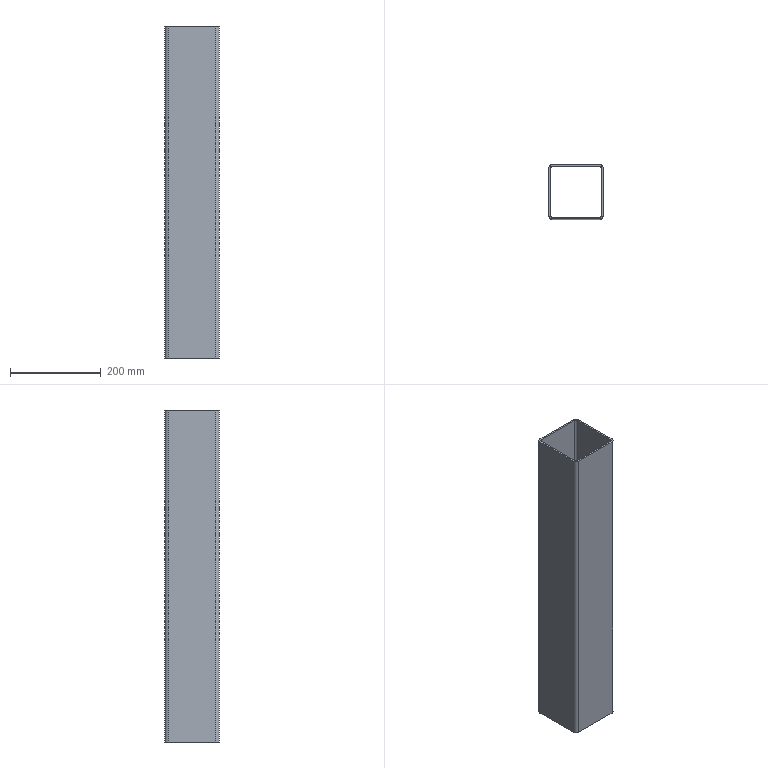Part | SolidWorks | features ICE 1, LibraryFeature 1 | 1 solid | 18 faces | box 120 x 120 x 730 mm | volume 1324801 mm3 | plane 10 | cylinder 8 | commonest cylinder face diameters 8 x4 16 x4
STEP:
#1=CARTESIAN_POINT('',(52.,60.,-365.));
#2=VERTEX_POINT('',#1);
#3=CARTESIAN_POINT('',(-52.,60.,-365.));
#4=VERTEX_POINT('',#3);
#5=CARTESIAN_POINT('',(0.,60.,-365.));
#6=DIRECTION('',(-1.,0.,0.));
#7=VECTOR('',#6,1000.);
#8=LINE('',#5,#7);
#9=EDGE_CURVE('',#2,#4,#8,.T.);
#10=ORIENTED_EDGE('',*,*,#9,.T.);
#11=CARTESIAN_POINT('',(-52.,60.,365.));
#12=VERTEX_POINT('',#11);
#13=CARTESIAN_POINT('',(-52.,60.,365.));
#14=DIRECTION('',(0.,0.,-1.));
#15=VECTOR('',#14,1000.);
#16=LINE('',#13,#15);
#17=EDGE_CURVE('',#12,#4,#16,.T.);
#18=ORIENTED_EDGE('',*,*,#17,.F.);
#19=CARTESIAN_POINT('',(52.,60.,365.));
#20=VERTEX_POINT('',#19);
#21=CARTESIAN_POINT('',(0.,60.,365.));
#22=DIRECTION('',(-1.,0.,0.));
#23=VECTOR('',#22,1000.);
#24=LINE('',#21,#23);
#25=EDGE_CURVE('',#20,#12,#24,.T.);
#26=ORIENTED_EDGE('',*,*,#25,.F.);
#27=CARTESIAN_POINT('',(52.,60.,365.));
#28=DIRECTION('',(0.,0.,-1.));
#29=VECTOR('',#28,1000.);
#30=LINE('',#27,#29);
#31=EDGE_CURVE('',#20,#2,#30,.T.);
#32=ORIENTED_EDGE('',*,*,#31,.T.);
#33=EDGE_LOOP('',(#10,#18,#26,#32));
#34=FACE_OUTER_BOUND('',#33,.T.);
#35=CARTESIAN_POINT('',(0.,60.,365.));
#36=DIRECTION('',(0.,-1.,0.));
#37=DIRECTION('',(0.,0.,-1.));
#38=AXIS2_PLACEMENT_3D('',#35,#36,#37);
#39=PLANE('',#38);
#40=ADVANCED_FACE('',(#34),#39,.F.);
#41=CARTESIAN_POINT('',(-60.,52.,-365.));
#42=VERTEX_POINT('',#41);
#43=CARTESIAN_POINT('',(-52.,52.,-365.));
#44=DIRECTION('',(0.,0.,1.));
#45=DIRECTION('',(1.,0.,0.));
#46=AXIS2_PLACEMENT_3D('',#43,#44,#45);
#47=CIRCLE('',#46,8.);
#48=EDGE_CURVE('',#4,#42,#47,.T.);
#49=ORIENTED_EDGE('',*,*,#48,.T.);
#50=CARTESIAN_POINT('',(-60.,52.,365.));
#51=VERTEX_POINT('',#50);
#52=CARTESIAN_POINT('',(-60.,52.,365.));
#53=DIRECTION('',(0.,0.,-1.));
#54=VECTOR('',#53,1000.);
#55=LINE('',#52,#54);
#56=EDGE_CURVE('',#51,#42,#55,.T.);
#57=ORIENTED_EDGE('',*,*,#56,.F.);
#58=CARTESIAN_POINT('',(-52.,52.,365.));
#59=DIRECTION('',(0.,0.,1.));
#60=DIRECTION('',(1.,0.,0.));
#61=AXIS2_PLACEMENT_3D('',#58,#59,#60);
#62=CIRCLE('',#61,8.);
#63=EDGE_CURVE('',#12,#51,#62,.T.);
#64=ORIENTED_EDGE('',*,*,#63,.F.);
#65=ORIENTED_EDGE('',*,*,#17,.T.);
#66=EDGE_LOOP('',(#49,#57,#64,#65));
#67=FACE_OUTER_BOUND('',#66,.T.);
#68=CARTESIAN_POINT('',(-52.,52.,365.));
#69=DIRECTION('',(0.,0.,-1.));
#70=DIRECTION('',(-1.,0.,0.));
#71=AXIS2_PLACEMENT_3D('',#68,#69,#70);
#72=CYLINDRICAL_SURFACE('',#71,8.);
#73=ADVANCED_FACE('',(#67),#72,.T.);
#74=CARTESIAN_POINT('',(-60.,-52.,-365.));
#75=VERTEX_POINT('',#74);
#76=CARTESIAN_POINT('',(-60.,0.,-365.));
#77=DIRECTION('',(0.,1.,0.));
#78=VECTOR('',#77,1000.);
#79=LINE('',#76,#78);
#80=EDGE_CURVE('',#75,#42,#79,.T.);
#81=ORIENTED_EDGE('',*,*,#80,.F.);
#82=CARTESIAN_POINT('',(-60.,-52.,365.));
#83=VERTEX_POINT('',#82);
#84=CARTESIAN_POINT('',(-60.,-52.,365.));
#85=DIRECTION('',(0.,0.,-1.));
#86=VECTOR('',#85,1000.);
#87=LINE('',#84,#86);
#88=EDGE_CURVE('',#83,#75,#87,.T.);
#89=ORIENTED_EDGE('',*,*,#88,.F.);
#90=CARTESIAN_POINT('',(-60.,0.,365.));
#91=DIRECTION('',(0.,1.,0.));
#92=VECTOR('',#91,1000.);
#93=LINE('',#90,#92);
#94=EDGE_CURVE('',#83,#51,#93,.T.);
#95=ORIENTED_EDGE('',*,*,#94,.T.);
#96=ORIENTED_EDGE('',*,*,#56,.T.);
#97=EDGE_LOOP('',(#81,#89,#95,#96));
#98=FACE_OUTER_BOUND('',#97,.T.);
#99=CARTESIAN_POINT('',(-60.,0.,365.));
#100=DIRECTION('',(-1.,0.,0.));
#101=DIRECTION('',(0.,0.,1.));
#102=AXIS2_PLACEMENT_3D('',#99,#100,#101);
#103=PLANE('',#102);
#104=ADVANCED_FACE('',(#98),#103,.T.);
#105=CARTESIAN_POINT('',(-52.,-60.,-365.));
#106=VERTEX_POINT('',#105);
#107=CARTESIAN_POINT('',(-52.,-52.,-365.));
#108=DIRECTION('',(0.,0.,1.));
#109=DIRECTION('',(1.,0.,0.));
#110=AXIS2_PLACEMENT_3D('',#107,#108,#109);
#111=CIRCLE('',#110,8.);
#112=EDGE_CURVE('',#75,#106,#111,.T.);
#113=ORIENTED_EDGE('',*,*,#112,.T.);
#114=CARTESIAN_POINT('',(-52.,-60.,365.));
#115=VERTEX_POINT('',#114);
#116=CARTESIAN_POINT('',(-52.,-60.,365.));
#117=DIRECTION('',(0.,0.,-1.));
#118=VECTOR('',#117,1000.);
#119=LINE('',#116,#118);
#120=EDGE_CURVE('',#115,#106,#119,.T.);
#121=ORIENTED_EDGE('',*,*,#120,.F.);
#122=CARTESIAN_POINT('',(-52.,-52.,365.));
#123=DIRECTION('',(0.,0.,1.));
#124=DIRECTION('',(1.,0.,0.));
#125=AXIS2_PLACEMENT_3D('',#122,#123,#124);
#126=CIRCLE('',#125,8.);
#127=EDGE_CURVE('',#83,#115,#126,.T.);
#128=ORIENTED_EDGE('',*,*,#127,.F.);
#129=ORIENTED_EDGE('',*,*,#88,.T.);
#130=EDGE_LOOP('',(#113,#121,#128,#129));
#131=FACE_OUTER_BOUND('',#130,.T.);
#132=CARTESIAN_POINT('',(-52.,-52.,365.));
#133=DIRECTION('',(0.,0.,-1.));
#134=DIRECTION('',(-1.,0.,0.));
#135=AXIS2_PLACEMENT_3D('',#132,#133,#134);
#136=CYLINDRICAL_SURFACE('',#135,8.);
#137=ADVANCED_FACE('',(#131),#136,.T.);
#138=CARTESIAN_POINT('',(52.,-60.,-365.));
#139=VERTEX_POINT('',#138);
#140=CARTESIAN_POINT('',(0.,-60.,-365.));
#141=DIRECTION('',(1.,0.,0.));
#142=VECTOR('',#141,1000.);
#143=LINE('',#140,#142);
#144=EDGE_CURVE('',#106,#139,#143,.T.);
#145=ORIENTED_EDGE('',*,*,#144,.T.);
#146=CARTESIAN_POINT('',(52.,-60.,365.));
#147=VERTEX_POINT('',#146);
#148=CARTESIAN_POINT('',(52.,-60.,365.));
#149=DIRECTION('',(0.,0.,-1.));
#150=VECTOR('',#149,1000.);
#151=LINE('',#148,#150);
#152=EDGE_CURVE('',#147,#139,#151,.T.);
#153=ORIENTED_EDGE('',*,*,#152,.F.);
#154=CARTESIAN_POINT('',(0.,-60.,365.));
#155=DIRECTION('',(1.,0.,0.));
#156=VECTOR('',#155,1000.);
#157=LINE('',#154,#156);
#158=EDGE_CURVE('',#115,#147,#157,.T.);
#159=ORIENTED_EDGE('',*,*,#158,.F.);
#160=ORIENTED_EDGE('',*,*,#120,.T.);
#161=EDGE_LOOP('',(#145,#153,#159,#160));
#162=FACE_OUTER_BOUND('',#161,.T.);
#163=CARTESIAN_POINT('',(0.,-60.,365.));
#164=DIRECTION('',(0.,1.,0.));
#165=DIRECTION('',(0.,0.,1.));
#166=AXIS2_PLACEMENT_3D('',#163,#164,#165);
#167=PLANE('',#166);
#168=ADVANCED_FACE('',(#162),#167,.F.);
#169=CARTESIAN_POINT('',(60.,-52.,-365.));
#170=VERTEX_POINT('',#169);
#171=CARTESIAN_POINT('',(52.,-52.,-365.));
#172=DIRECTION('',(0.,0.,1.));
#173=DIRECTION('',(1.,0.,0.));
#174=AXIS2_PLACEMENT_3D('',#171,#172,#173);
#175=CIRCLE('',#174,8.);
#176=EDGE_CURVE('',#139,#170,#175,.T.);
#177=ORIENTED_EDGE('',*,*,#176,.T.);
#178=CARTESIAN_POINT('',(60.,-52.,365.));
#179=VERTEX_POINT('',#178);
#180=CARTESIAN_POINT('',(60.,-52.,365.));
#181=DIRECTION('',(0.,0.,-1.));
#182=VECTOR('',#181,1000.);
#183=LINE('',#180,#182);
#184=EDGE_CURVE('',#179,#170,#183,.T.);
#185=ORIENTED_EDGE('',*,*,#184,.F.);
#186=CARTESIAN_POINT('',(52.,-52.,365.));
#187=DIRECTION('',(0.,0.,1.));
#188=DIRECTION('',(1.,0.,0.));
#189=AXIS2_PLACEMENT_3D('',#186,#187,#188);
#190=CIRCLE('',#189,8.);
#191=EDGE_CURVE('',#147,#179,#190,.T.);
#192=ORIENTED_EDGE('',*,*,#191,.F.);
#193=ORIENTED_EDGE('',*,*,#152,.T.);
#194=EDGE_LOOP('',(#177,#185,#192,#193));
#195=FACE_OUTER_BOUND('',#194,.T.);
#196=CARTESIAN_POINT('',(52.,-52.,365.));
#197=DIRECTION('',(0.,0.,-1.));
#198=DIRECTION('',(-1.,0.,0.));
#199=AXIS2_PLACEMENT_3D('',#196,#197,#198);
#200=CYLINDRICAL_SURFACE('',#199,8.);
#201=ADVANCED_FACE('',(#195),#200,.T.);
#202=CARTESIAN_POINT('',(60.,52.,-365.));
#203=VERTEX_POINT('',#202);
#204=CARTESIAN_POINT('',(60.,0.,-365.));
#205=DIRECTION('',(0.,-1.,0.));
#206=VECTOR('',#205,1000.);
#207=LINE('',#204,#206);
#208=EDGE_CURVE('',#203,#170,#207,.T.);
#209=ORIENTED_EDGE('',*,*,#208,.F.);
#210=CARTESIAN_POINT('',(60.,52.,365.));
#211=VERTEX_POINT('',#210);
#212=CARTESIAN_POINT('',(60.,52.,365.));
#213=DIRECTION('',(0.,0.,-1.));
#214=VECTOR('',#213,1000.);
#215=LINE('',#212,#214);
#216=EDGE_CURVE('',#211,#203,#215,.T.);
#217=ORIENTED_EDGE('',*,*,#216,.F.);
#218=CARTESIAN_POINT('',(60.,0.,365.));
#219=DIRECTION('',(0.,-1.,0.));
#220=VECTOR('',#219,1000.);
#221=LINE('',#218,#220);
#222=EDGE_CURVE('',#211,#179,#221,.T.);
#223=ORIENTED_EDGE('',*,*,#222,.T.);
#224=ORIENTED_EDGE('',*,*,#184,.T.);
#225=EDGE_LOOP('',(#209,#217,#223,#224));
#226=FACE_OUTER_BOUND('',#225,.T.);
#227=CARTESIAN_POINT('',(60.,0.,365.));
#228=DIRECTION('',(1.,0.,0.));
#229=DIRECTION('',(0.,0.,-1.));
#230=AXIS2_PLACEMENT_3D('',#227,#228,#229);
#231=PLANE('',#230);
#232=ADVANCED_FACE('',(#226),#231,.T.);
#233=CARTESIAN_POINT('',(-56.,-52.,-365.));
#234=VERTEX_POINT('',#233);
#235=CARTESIAN_POINT('',(-52.,-56.,-365.));
#236=VERTEX_POINT('',#235);
#237=CARTESIAN_POINT('',(-52.,-52.,-365.));
#238=DIRECTION('',(0.,0.,1.));
#239=DIRECTION('',(1.,0.,0.));
#240=AXIS2_PLACEMENT_3D('',#237,#238,#239);
#241=CIRCLE('',#240,4.);
#242=EDGE_CURVE('',#234,#236,#241,.T.);
#243=ORIENTED_EDGE('',*,*,#242,.F.);
#244=CARTESIAN_POINT('',(-56.,-52.,365.));
#245=VERTEX_POINT('',#244);
#246=CARTESIAN_POINT('',(-56.,-52.,365.));
#247=DIRECTION('',(0.,0.,-1.));
#248=VECTOR('',#247,1000.);
#249=LINE('',#246,#248);
#250=EDGE_CURVE('',#245,#234,#249,.T.);
#251=ORIENTED_EDGE('',*,*,#250,.F.);
#252=CARTESIAN_POINT('',(-52.,-56.,365.));
#253=VERTEX_POINT('',#252);
#254=CARTESIAN_POINT('',(-52.,-52.,365.));
#255=DIRECTION('',(0.,0.,1.));
#256=DIRECTION('',(1.,0.,0.));
#257=AXIS2_PLACEMENT_3D('',#254,#255,#256);
#258=CIRCLE('',#257,4.);
#259=EDGE_CURVE('',#245,#253,#258,.T.);
#260=ORIENTED_EDGE('',*,*,#259,.T.);
#261=CARTESIAN_POINT('',(-52.,-56.,365.));
#262=DIRECTION('',(0.,0.,-1.));
#263=VECTOR('',#262,1000.);
#264=LINE('',#261,#263);
#265=EDGE_CURVE('',#253,#236,#264,.T.);
#266=ORIENTED_EDGE('',*,*,#265,.T.);
#267=EDGE_LOOP('',(#243,#251,#260,#266));
#268=FACE_OUTER_BOUND('',#267,.T.);
#269=CARTESIAN_POINT('',(-52.,-52.,365.));
#270=DIRECTION('',(0.,0.,-1.));
#271=DIRECTION('',(-1.,0.,0.));
#272=AXIS2_PLACEMENT_3D('',#269,#270,#271);
#273=CYLINDRICAL_SURFACE('',#272,4.);
#274=ADVANCED_FACE('',(#268),#273,.F.);
#275=CARTESIAN_POINT('',(-56.,52.,-365.));
#276=VERTEX_POINT('',#275);
#277=CARTESIAN_POINT('',(-56.,0.,-365.));
#278=DIRECTION('',(0.,1.,0.));
#279=VECTOR('',#278,1000.);
#280=LINE('',#277,#279);
#281=EDGE_CURVE('',#234,#276,#280,.T.);
#282=ORIENTED_EDGE('',*,*,#281,.T.);
#283=CARTESIAN_POINT('',(-56.,52.,365.));
#284=VERTEX_POINT('',#283);
#285=CARTESIAN_POINT('',(-56.,52.,365.));
#286=DIRECTION('',(0.,0.,-1.));
#287=VECTOR('',#286,1000.);
#288=LINE('',#285,#287);
#289=EDGE_CURVE('',#284,#276,#288,.T.);
#290=ORIENTED_EDGE('',*,*,#289,.F.);
#291=CARTESIAN_POINT('',(-56.,0.,365.));
#292=DIRECTION('',(0.,1.,0.));
#293=VECTOR('',#292,1000.);
#294=LINE('',#291,#293);
#295=EDGE_CURVE('',#245,#284,#294,.T.);
#296=ORIENTED_EDGE('',*,*,#295,.F.);
#297=ORIENTED_EDGE('',*,*,#250,.T.);
#298=EDGE_LOOP('',(#282,#290,#296,#297));
#299=FACE_OUTER_BOUND('',#298,.T.);
#300=CARTESIAN_POINT('',(-56.,0.,365.));
#301=DIRECTION('',(-1.,0.,0.));
#302=DIRECTION('',(0.,0.,1.));
#303=AXIS2_PLACEMENT_3D('',#300,#301,#302);
#304=PLANE('',#303);
#305=ADVANCED_FACE('',(#299),#304,.F.);
#306=CARTESIAN_POINT('',(-52.,56.,-365.));
#307=VERTEX_POINT('',#306);
#308=CARTESIAN_POINT('',(-52.,52.,-365.));
#309=DIRECTION('',(0.,0.,1.));
#310=DIRECTION('',(1.,0.,0.));
#311=AXIS2_PLACEMENT_3D('',#308,#309,#310);
#312=CIRCLE('',#311,4.);
#313=EDGE_CURVE('',#307,#276,#312,.T.);
#314=ORIENTED_EDGE('',*,*,#313,.F.);
#315=CARTESIAN_POINT('',(-52.,56.,365.));
#316=VERTEX_POINT('',#315);
#317=CARTESIAN_POINT('',(-52.,56.,365.));
#318=DIRECTION('',(0.,0.,-1.));
#319=VECTOR('',#318,1000.);
#320=LINE('',#317,#319);
#321=EDGE_CURVE('',#316,#307,#320,.T.);
#322=ORIENTED_EDGE('',*,*,#321,.F.);
#323=CARTESIAN_POINT('',(-52.,52.,365.));
#324=DIRECTION('',(0.,0.,1.));
#325=DIRECTION('',(1.,0.,0.));
#326=AXIS2_PLACEMENT_3D('',#323,#324,#325);
#327=CIRCLE('',#326,4.);
#328=EDGE_CURVE('',#316,#284,#327,.T.);
#329=ORIENTED_EDGE('',*,*,#328,.T.);
#330=ORIENTED_EDGE('',*,*,#289,.T.);
#331=EDGE_LOOP('',(#314,#322,#329,#330));
#332=FACE_OUTER_BOUND('',#331,.T.);
#333=CARTESIAN_POINT('',(-52.,52.,365.));
#334=DIRECTION('',(0.,0.,-1.));
#335=DIRECTION('',(-1.,0.,0.));
#336=AXIS2_PLACEMENT_3D('',#333,#334,#335);
#337=CYLINDRICAL_SURFACE('',#336,4.);
#338=ADVANCED_FACE('',(#332),#337,.F.);
#339=CARTESIAN_POINT('',(52.,56.,-365.));
#340=VERTEX_POINT('',#339);
#341=CARTESIAN_POINT('',(0.,56.,-365.));
#342=DIRECTION('',(-1.,0.,0.));
#343=VECTOR('',#342,1000.);
#344=LINE('',#341,#343);
#345=EDGE_CURVE('',#340,#307,#344,.T.);
#346=ORIENTED_EDGE('',*,*,#345,.F.);
#347=CARTESIAN_POINT('',(52.,56.,365.));
#348=VERTEX_POINT('',#347);
#349=CARTESIAN_POINT('',(52.,56.,365.));
#350=DIRECTION('',(0.,0.,-1.));
#351=VECTOR('',#350,1000.);
#352=LINE('',#349,#351);
#353=EDGE_CURVE('',#348,#340,#352,.T.);
#354=ORIENTED_EDGE('',*,*,#353,.F.);
#355=CARTESIAN_POINT('',(0.,56.,365.));
#356=DIRECTION('',(-1.,0.,0.));
#357=VECTOR('',#356,1000.);
#358=LINE('',#355,#357);
#359=EDGE_CURVE('',#348,#316,#358,.T.);
#360=ORIENTED_EDGE('',*,*,#359,.T.);
#361=ORIENTED_EDGE('',*,*,#321,.T.);
#362=EDGE_LOOP('',(#346,#354,#360,#361));
#363=FACE_OUTER_BOUND('',#362,.T.);
#364=CARTESIAN_POINT('',(0.,56.,365.));
#365=DIRECTION('',(0.,-1.,0.));
#366=DIRECTION('',(0.,0.,-1.));
#367=AXIS2_PLACEMENT_3D('',#364,#365,#366);
#368=PLANE('',#367);
#369=ADVANCED_FACE('',(#363),#368,.T.);
#370=CARTESIAN_POINT('',(56.,52.,-365.));
#371=VERTEX_POINT('',#370);
#372=CARTESIAN_POINT('',(52.,52.,-365.));
#373=DIRECTION('',(0.,0.,1.));
#374=DIRECTION('',(1.,0.,0.));
#375=AXIS2_PLACEMENT_3D('',#372,#373,#374);
#376=CIRCLE('',#375,4.);
#377=EDGE_CURVE('',#371,#340,#376,.T.);
#378=ORIENTED_EDGE('',*,*,#377,.F.);
#379=CARTESIAN_POINT('',(56.,52.,365.));
#380=VERTEX_POINT('',#379);
#381=CARTESIAN_POINT('',(56.,52.,365.));
#382=DIRECTION('',(0.,0.,-1.));
#383=VECTOR('',#382,1000.);
#384=LINE('',#381,#383);
#385=EDGE_CURVE('',#380,#371,#384,.T.);
#386=ORIENTED_EDGE('',*,*,#385,.F.);
#387=CARTESIAN_POINT('',(52.,52.,365.));
#388=DIRECTION('',(0.,0.,1.));
#389=DIRECTION('',(1.,0.,0.));
#390=AXIS2_PLACEMENT_3D('',#387,#388,#389);
#391=CIRCLE('',#390,4.);
#392=EDGE_CURVE('',#380,#348,#391,.T.);
#393=ORIENTED_EDGE('',*,*,#392,.T.);
#394=ORIENTED_EDGE('',*,*,#353,.T.);
#395=EDGE_LOOP('',(#378,#386,#393,#394));
#396=FACE_OUTER_BOUND('',#395,.T.);
#397=CARTESIAN_POINT('',(52.,52.,365.));
#398=DIRECTION('',(0.,0.,-1.));
#399=DIRECTION('',(-1.,0.,0.));
#400=AXIS2_PLACEMENT_3D('',#397,#398,#399);
#401=CYLINDRICAL_SURFACE('',#400,4.);
#402=ADVANCED_FACE('',(#396),#401,.F.);
#403=CARTESIAN_POINT('',(56.,-52.,-365.));
#404=VERTEX_POINT('',#403);
#405=CARTESIAN_POINT('',(56.,0.,-365.));
#406=DIRECTION('',(0.,-1.,0.));
#407=VECTOR('',#406,1000.);
#408=LINE('',#405,#407);
#409=EDGE_CURVE('',#371,#404,#408,.T.);
#410=ORIENTED_EDGE('',*,*,#409,.T.);
#411=CARTESIAN_POINT('',(56.,-52.,365.));
#412=VERTEX_POINT('',#411);
#413=CARTESIAN_POINT('',(56.,-52.,365.));
#414=DIRECTION('',(0.,0.,-1.));
#415=VECTOR('',#414,1000.);
#416=LINE('',#413,#415);
#417=EDGE_CURVE('',#412,#404,#416,.T.);
#418=ORIENTED_EDGE('',*,*,#417,.F.);
#419=CARTESIAN_POINT('',(56.,0.,365.));
#420=DIRECTION('',(0.,-1.,0.));
#421=VECTOR('',#420,1000.);
#422=LINE('',#419,#421);
#423=EDGE_CURVE('',#380,#412,#422,.T.);
#424=ORIENTED_EDGE('',*,*,#423,.F.);
#425=ORIENTED_EDGE('',*,*,#385,.T.);
#426=EDGE_LOOP('',(#410,#418,#424,#425));
#427=FACE_OUTER_BOUND('',#426,.T.);
#428=CARTESIAN_POINT('',(56.,0.,365.));
#429=DIRECTION('',(1.,0.,0.));
#430=DIRECTION('',(0.,0.,-1.));
#431=AXIS2_PLACEMENT_3D('',#428,#429,#430);
#432=PLANE('',#431);
#433=ADVANCED_FACE('',(#427),#432,.F.);
#434=CARTESIAN_POINT('',(52.,-56.,-365.));
#435=VERTEX_POINT('',#434);
#436=CARTESIAN_POINT('',(52.,-52.,-365.));
#437=DIRECTION('',(0.,0.,1.));
#438=DIRECTION('',(1.,0.,0.));
#439=AXIS2_PLACEMENT_3D('',#436,#437,#438);
#440=CIRCLE('',#439,4.);
#441=EDGE_CURVE('',#435,#404,#440,.T.);
#442=ORIENTED_EDGE('',*,*,#441,.F.);
#443=CARTESIAN_POINT('',(52.,-56.,365.));
#444=VERTEX_POINT('',#443);
#445=CARTESIAN_POINT('',(52.,-56.,365.));
#446=DIRECTION('',(0.,0.,-1.));
#447=VECTOR('',#446,1000.);
#448=LINE('',#445,#447);
#449=EDGE_CURVE('',#444,#435,#448,.T.);
#450=ORIENTED_EDGE('',*,*,#449,.F.);
#451=CARTESIAN_POINT('',(52.,-52.,365.));
#452=DIRECTION('',(0.,0.,1.));
#453=DIRECTION('',(1.,0.,0.));
#454=AXIS2_PLACEMENT_3D('',#451,#452,#453);
#455=CIRCLE('',#454,4.);
#456=EDGE_CURVE('',#444,#412,#455,.T.);
#457=ORIENTED_EDGE('',*,*,#456,.T.);
#458=ORIENTED_EDGE('',*,*,#417,.T.);
#459=EDGE_LOOP('',(#442,#450,#457,#458));
#460=FACE_OUTER_BOUND('',#459,.T.);
#461=CARTESIAN_POINT('',(52.,-52.,365.));
#462=DIRECTION('',(0.,0.,-1.));
#463=DIRECTION('',(-1.,0.,0.));
#464=AXIS2_PLACEMENT_3D('',#461,#462,#463);
#465=CYLINDRICAL_SURFACE('',#464,4.);
#466=ADVANCED_FACE('',(#460),#465,.F.);
#467=CARTESIAN_POINT('',(0.,-56.,-365.));
#468=DIRECTION('',(1.,0.,0.));
#469=VECTOR('',#468,1000.);
#470=LINE('',#467,#469);
#471=EDGE_CURVE('',#236,#435,#470,.T.);
#472=ORIENTED_EDGE('',*,*,#471,.F.);
#473=ORIENTED_EDGE('',*,*,#265,.F.);
#474=CARTESIAN_POINT('',(0.,-56.,365.));
#475=DIRECTION('',(1.,0.,0.));
#476=VECTOR('',#475,1000.);
#477=LINE('',#474,#476);
#478=EDGE_CURVE('',#253,#444,#477,.T.);
#479=ORIENTED_EDGE('',*,*,#478,.T.);
#480=ORIENTED_EDGE('',*,*,#449,.T.);
#481=EDGE_LOOP('',(#472,#473,#479,#480));
#482=FACE_OUTER_BOUND('',#481,.T.);
#483=CARTESIAN_POINT('',(0.,-56.,365.));
#484=DIRECTION('',(0.,1.,0.));
#485=DIRECTION('',(0.,0.,1.));
#486=AXIS2_PLACEMENT_3D('',#483,#484,#485);
#487=PLANE('',#486);
#488=ADVANCED_FACE('',(#482),#487,.T.);
#489=CARTESIAN_POINT('',(52.,52.,-365.));
#490=DIRECTION('',(0.,0.,1.));
#491=DIRECTION('',(1.,0.,0.));
#492=AXIS2_PLACEMENT_3D('',#489,#490,#491);
#493=CIRCLE('',#492,8.);
#494=EDGE_CURVE('',#203,#2,#493,.T.);
#495=ORIENTED_EDGE('',*,*,#494,.T.);
#496=ORIENTED_EDGE('',*,*,#31,.F.);
#497=CARTESIAN_POINT('',(52.,52.,365.));
#498=DIRECTION('',(0.,0.,1.));
#499=DIRECTION('',(1.,0.,0.));
#500=AXIS2_PLACEMENT_3D('',#497,#498,#499);
#501=CIRCLE('',#500,8.);
#502=EDGE_CURVE('',#211,#20,#501,.T.);
#503=ORIENTED_EDGE('',*,*,#502,.F.);
#504=ORIENTED_EDGE('',*,*,#216,.T.);
#505=EDGE_LOOP('',(#495,#496,#503,#504));
#506=FACE_OUTER_BOUND('',#505,.T.);
#507=CARTESIAN_POINT('',(52.,52.,365.));
#508=DIRECTION('',(0.,0.,-1.));
#509=DIRECTION('',(-1.,0.,0.));
#510=AXIS2_PLACEMENT_3D('',#507,#508,#509);
#511=CYLINDRICAL_SURFACE('',#510,8.);
#512=ADVANCED_FACE('',(#506),#511,.T.);
#513=ORIENTED_EDGE('',*,*,#259,.F.);
#514=ORIENTED_EDGE('',*,*,#295,.T.);
#515=ORIENTED_EDGE('',*,*,#328,.F.);
#516=ORIENTED_EDGE('',*,*,#359,.F.);
#517=ORIENTED_EDGE('',*,*,#392,.F.);
#518=ORIENTED_EDGE('',*,*,#423,.T.);
#519=ORIENTED_EDGE('',*,*,#456,.F.);
#520=ORIENTED_EDGE('',*,*,#478,.F.);
#521=EDGE_LOOP('',(#513,#514,#515,#516,#517,#518,#519,#520));
#522=FACE_BOUND('',#521,.T.);
#523=ORIENTED_EDGE('',*,*,#25,.T.);
#524=ORIENTED_EDGE('',*,*,#63,.T.);
#525=ORIENTED_EDGE('',*,*,#94,.F.);
#526=ORIENTED_EDGE('',*,*,#127,.T.);
#527=ORIENTED_EDGE('',*,*,#158,.T.);
#528=ORIENTED_EDGE('',*,*,#191,.T.);
#529=ORIENTED_EDGE('',*,*,#222,.F.);
#530=ORIENTED_EDGE('',*,*,#502,.T.);
#531=EDGE_LOOP('',(#523,#524,#525,#526,#527,#528,#529,#530));
#532=FACE_OUTER_BOUND('',#531,.T.);
#533=CARTESIAN_POINT('',(0.,0.,365.));
#534=DIRECTION('',(0.,0.,1.));
#535=DIRECTION('',(1.,0.,0.));
#536=AXIS2_PLACEMENT_3D('',#533,#534,#535);
#537=PLANE('',#536);
#538=ADVANCED_FACE('',(#522,#532),#537,.T.);
#539=ORIENTED_EDGE('',*,*,#242,.T.);
#540=ORIENTED_EDGE('',*,*,#471,.T.);
#541=ORIENTED_EDGE('',*,*,#441,.T.);
#542=ORIENTED_EDGE('',*,*,#409,.F.);
#543=ORIENTED_EDGE('',*,*,#377,.T.);
#544=ORIENTED_EDGE('',*,*,#345,.T.);
#545=ORIENTED_EDGE('',*,*,#313,.T.);
#546=ORIENTED_EDGE('',*,*,#281,.F.);
#547=EDGE_LOOP('',(#539,#540,#541,#542,#543,#544,#545,#546));
#548=FACE_BOUND('',#547,.T.);
#549=ORIENTED_EDGE('',*,*,#9,.F.);
#550=ORIENTED_EDGE('',*,*,#494,.F.);
#551=ORIENTED_EDGE('',*,*,#208,.T.);
#552=ORIENTED_EDGE('',*,*,#176,.F.);
#553=ORIENTED_EDGE('',*,*,#144,.F.);
#554=ORIENTED_EDGE('',*,*,#112,.F.);
#555=ORIENTED_EDGE('',*,*,#80,.T.);
#556=ORIENTED_EDGE('',*,*,#48,.F.);
#557=EDGE_LOOP('',(#549,#550,#551,#552,#553,#554,#555,#556));
#558=FACE_OUTER_BOUND('',#557,.T.);
#559=CARTESIAN_POINT('',(0.,0.,-365.));
#560=DIRECTION('',(0.,0.,1.));
#561=DIRECTION('',(1.,0.,0.));
#562=AXIS2_PLACEMENT_3D('',#559,#560,#561);
#563=PLANE('',#562);
#564=ADVANCED_FACE('',(#548,#558),#563,.F.);
#565=CLOSED_SHELL('',(#40,#73,#104,#137,#168,#201,#232,#274,#305,#338,#369,#402,#433,#466,#488,#512,#538,#564));
#566=MANIFOLD_SOLID_BREP('',#565);
#567=CARTESIAN_POINT('',(0.,0.,0.));
#568=DIRECTION('',(0.,0.,1.));
#569=DIRECTION('',(1.,0.,0.));
#570=AXIS2_PLACEMENT_3D('',#567,#568,#569);
#571=(LENGTH_UNIT()NAMED_UNIT(*)SI_UNIT(.MILLI.,.METRE.));
#572=UNCERTAINTY_MEASURE_WITH_UNIT(LENGTH_MEASURE(0.00001),#571,'','');
#573=(NAMED_UNIT(*)PLANE_ANGLE_UNIT()SI_UNIT($,.RADIAN.));
#574=(NAMED_UNIT(*)SI_UNIT($,.STERADIAN.)SOLID_ANGLE_UNIT());
#575=(GEOMETRIC_REPRESENTATION_CONTEXT(3)GLOBAL_UNCERTAINTY_ASSIGNED_CONTEXT((#572))GLOBAL_UNIT_ASSIGNED_CONTEXT((#571,#573,#574))REPRESENTATION_CONTEXT('',''));
#576=ADVANCED_BREP_SHAPE_REPRESENTATION('',(#566,#570),#575);